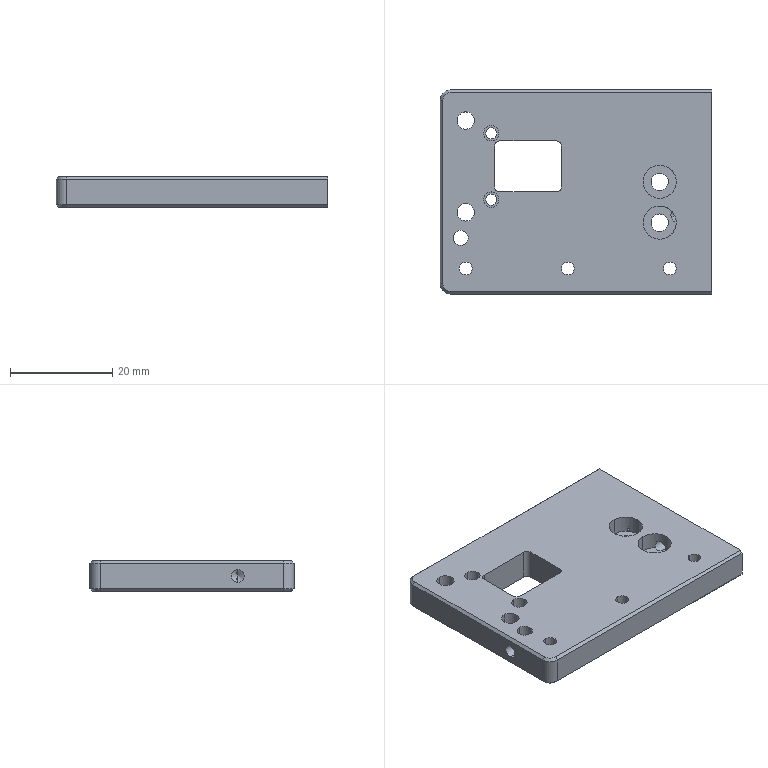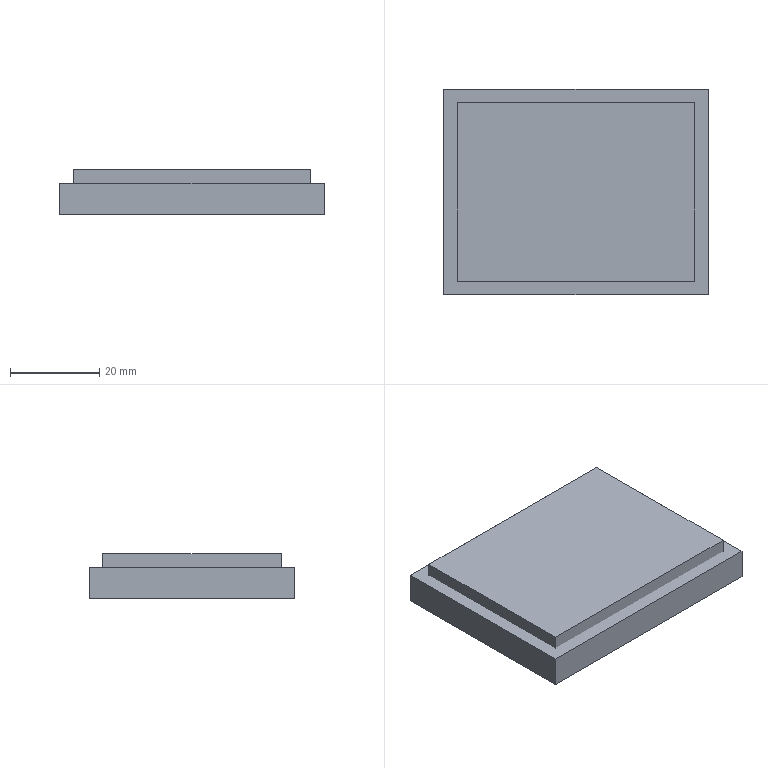CAM job | NX | 3+2 milling, drilling | part box 53.2 x 40 x 6 mm | stock box 59.2 x 46 x 10 mm
Tools:
number,name,description,diameter,corner_radius,flute_length,length,flutes
1,D50,Milling Tool-5 Parameters,50.0,0.0,50.0,75.0,2
7,D6A45,Milling Tool-5 Parameters,6.0,0.0,3.0,3.0,2
13,3.4ZT,Drilling Tool,3.4,0.0,35.0,50.0,2
11,2.5ZT,Drilling Tool,2.5,0.0,35.0,50.0,2
12,2.2ZT,Drilling Tool,2.2,0.0,35.0,50.0,2
10,D10,Milling Tool-5 Parameters,10.0,0.0,50.0,75.0,2
6,D6,Milling Tool-5 Parameters,6.0,0.0,50.0,75.0,2
4,D4,Milling Tool-5 Parameters,4.0,0.0,50.0,75.0,2
5,D2,Milling Tool-5 Parameters,2.0,0.0,50.0,75.0,2
Operations:
program,operation,operation_type,tool,method,geometry_group,spindle_rpm,surface_speed,feed_per_tooth,feed_cut,feed_plunge,cut_length_mm,path_length_mm,cut_time_min,machine_time_min
1-10-45-58毛胚-虎钳,FLOOR_WALL,VolumeBased25DMillingOperation,D50,METHOD,A,6500.0,1286.0,0.0962,1250.0,100.0,121.2,175.2,0.097,0.1024
1-10-45-58毛胚-虎钳,DRILLING_COPY_1,Operation,D6A45,METHOD,A,3000.0,56.0,0.0333,200.0,0.0,40.0,264.416,0.2,0.2224
1-10-45-58毛胚-虎钳,DRILLING_COPY_1_COPY_COPY_COPY_COPY,Operation,3.4ZT,METHOD,A,2000.0,21.0,0.0375,150.0,0.0,22.043,125.334,0.147,0.1573
1-10-45-58毛胚-虎钳,DRILLING_COPY_1_COPY_COPY_COPY_COPY_COPY,Operation,2.5ZT,METHOD,A,2000.0,15.0,0.0375,150.0,0.0,43.004,202.238,0.2867,0.3026
1-10-45-58毛胚-虎钳,DRILLING_COPY_1_COPY_COPY_COPY_COPY_COPY_COPY_COPY,Operation,2.2ZT,METHOD,A,2000.0,15.0,0.0375,150.0,0.0,21.322,118.986,0.1421,0.1519
1-10-45-58毛胚-虎钳,ZLEVEL_PROFILE,ZLevelMilling,D10,METHOD,A,7000.0,219.0,0.2143,3000.0,1000.0,1406.957,1469.957,0.5008,0.5071
1-10-45-58毛胚-虎钳,ZLEVEL_PROFILE_COPY,ZLevelMilling,D6,METHOD,A,7000.0,219.0,0.2143,3000.0,1000.0,310.101,373.101,0.1288,0.1351
1-10-45-58毛胚-虎钳,HOLE_MILLING,CylinderMilling,D4,METHOD,A,7000.0,131.0,0.1071,1500.0,100.0,227.914,361.714,0.1519,0.1653
1-10-45-58毛胚-虎钳,ZLEVEL_PROFILE_COPY_1,ZLevelMilling,D4,METHOD,A,7000.0,87.0,0.1071,1500.0,1000.0,289.284,660.942,0.2151,0.2523
1-10-45-58毛胚-虎钳,ZLEVEL_PROFILE_COPY_COPY_1_COPY_COPY_COPY_1,ZLevelMilling,D4,METHOD,A,7000.0,219.0,0.0714,1000.0,100.0,229.822,398.438,0.2298,0.2467
1-10-45-58毛胚-虎钳,ZLEVEL_PROFILE_COPY_1_COPY,ZLevelMilling,D2,METHOD,A,7000.0,43.0,0.0786,1100.0,1000.0,445.164,932.713,0.4108,0.4595
1-10-45-58毛胚-虎钳,HOLE_MILLING_COPY,CylinderMilling,D2,METHOD,A,7000.0,43.0,0.0786,1100.0,100.0,343.055,560.159,0.3119,0.3336
1-10-45-58毛胚-虎钳,ZLEVEL_PROFILE_COPY_1_COPY_COPY_COPY_COPY_2_COPY_COPY_1,ZLevelMilling,D6A45,METHOD,A,7000.0,131.0,0.0714,1000.0,1000.0,304.721,1296.217,0.3047,0.4039
1-10-45-58毛胚-虎钳,CUTTERCOMP5,CylinderMilling,D2,METHOD,A,7000.0,43.0,0.0607,850.0,100.0,66.487,283.591,0.0782,0.0999
2-10-45-58毛胚-虎钳,FLOOR_WALL_COPY,VolumeBased25DMillingOperation,D50,METHOD,B,6500.0,1286.0,0.0962,1250.0,100.0,460.8,992.401,0.3686,0.4218
2-10-45-58毛胚-虎钳,DRILLING_COPY_1_COPY,Operation,D6A45,METHOD,B,3000.0,56.0,0.0333,200.0,0.0,9.7,90.944,0.0485,0.0566
2-10-45-58毛胚-虎钳,DRILLING_COPY_1_COPY_COPY_COPY_COPY_COPY_1,Operation,3.4ZT,METHOD,B,2000.0,21.0,0.0375,150.0,0.0,22.043,115.63,0.147,0.1563
2-10-45-58毛胚-虎钳,HOLE_MILLING_COPY_1,CylinderMilling,D4,METHOD,B,7000.0,131.0,0.1071,1500.0,100.0,227.914,371.714,0.1519,0.1663
2-10-45-58毛胚-虎钳,DRILLING_COPY_1_COPY_COPY,Operation,D6A45,METHOD,B,3000.0,56.0,0.0333,200.0,0.0,8.4,93.142,0.042,0.0505
2-10-45-58毛胚-虎钳,ZLEVEL_PROFILE_COPY_1_COPY_COPY_COPY_COPY_2_COPY_COPY_1_COPY,ZLevelMilling,D6A45,METHOD,B,7000.0,131.0,0.0714,1000.0,1000.0,295.409,1165.721,0.2954,0.3824
3-10-45-58毛胚-虎钳,DRILLING_COPY_1_COPY_1,Operation,D6A45,METHOD,C,3000.0,56.0,0.0333,200.0,0.0,23.0,140.485,0.115,0.1267
3-10-45-58毛胚-虎钳,DRILLING_COPY_1_COPY_COPY_COPY_COPY_COPY_COPY,Operation,2.5ZT,METHOD,C,2000.0,15.0,0.0375,150.0,0.0,51.165,196.815,0.3411,0.3557
3-10-45-58毛胚-虎钳,ZLEVEL_PROFILE_1,ZLevelMilling,D2,METHOD,C,7000.0,65.0,0.0786,1100.0,1000.0,309.534,444.555,0.2854,0.2989
3-10-45-58毛胚-虎钳,ZLEVEL_PROFILE_COPY_1_COPY_COPY_COPY_COPY_2_COPY_COPY_1_1_COPY_1,ZLevelMilling,D6A45,METHOD,C,7000.0,131.0,0.0714,1000.0,1000.0,21.182,359.274,0.0212,0.055
3-10-45-58毛胚-虎钳,CUTTERCOMP5.,ZLevelMilling,D2,METHOD,C,7000.0,65.0,0.0786,1100.0,1000.0,48.64,188.225,0.0444,0.0583
4-10-45-58毛胚-虎钳,DRILLING_COPY_1_COPY_1_COPY,Operation,D6A45,METHOD,D,3000.0,56.0,0.0333,200.0,0.0,4.6,69.2,0.023,0.0295
4-10-45-58毛胚-虎钳,DRILLING_COPY_1_COPY_COPY_COPY_COPY_COPY_COPY_1_COPY,Operation,2.5ZT,METHOD,D,2000.0,15.0,0.0375,150.0,0.0,7.422,74.844,0.0495,0.0562